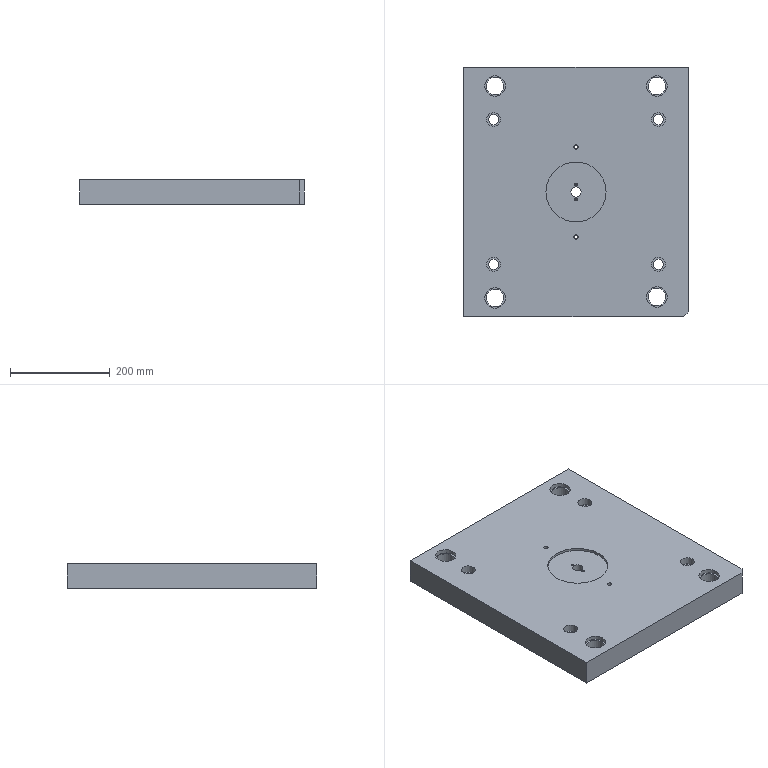Part | STEP file | SL2-MOLD_id730_xmt_txt | 1 solid | 46 faces | box 450 x 500 x 50 mm | volume 10885298 mm3 | cylinder 24 | plane 20 | cone 2 | commonest cylinder face diameters 20.5 x5 27.5 x4 35 x4 41 x4 5 x2 6 x2
STEP:
#1=CARTESIAN_POINT('',(-225.,-160.,136.));
#2=VERTEX_POINT('',#1);
#3=CARTESIAN_POINT('',(215.,-160.,136.));
#4=VERTEX_POINT('',#3);
#5=CARTESIAN_POINT('',(-130.,-160.,136.));
#6=DIRECTION('',(1.,0.,0.));
#7=VECTOR('',#6,1.);
#8=LINE('',#5,#7);
#9=EDGE_CURVE('',#2,#4,#8,.T.);
#10=ORIENTED_EDGE('',*,*,#9,.T.);
#11=CARTESIAN_POINT('',(215.,-160.,186.));
#12=VERTEX_POINT('',#11);
#13=CARTESIAN_POINT('',(215.,-160.,186.));
#14=DIRECTION('',(0.,0.,1.));
#15=VECTOR('',#14,1.);
#16=LINE('',#13,#15);
#17=EDGE_CURVE('',#4,#12,#16,.T.);
#18=ORIENTED_EDGE('',*,*,#17,.T.);
#19=CARTESIAN_POINT('',(-225.,-160.,186.));
#20=VERTEX_POINT('',#19);
#21=CARTESIAN_POINT('',(-130.,-160.,186.));
#22=DIRECTION('',(1.,0.,0.));
#23=VECTOR('',#22,1.);
#24=LINE('',#21,#23);
#25=EDGE_CURVE('',#20,#12,#24,.T.);
#26=ORIENTED_EDGE('',*,*,#25,.F.);
#27=CARTESIAN_POINT('',(-225.,-160.,186.));
#28=DIRECTION('',(0.,0.,-1.));
#29=VECTOR('',#28,1.);
#30=LINE('',#27,#29);
#31=EDGE_CURVE('',#20,#2,#30,.T.);
#32=ORIENTED_EDGE('',*,*,#31,.T.);
#33=EDGE_LOOP('',(#10,#18,#26,#32));
#34=FACE_OUTER_BOUND('',#33,.T.);
#35=CARTESIAN_POINT('',(-130.,-160.,186.));
#36=DIRECTION('',(0.,1.,0.));
#37=DIRECTION('',(0.,0.,1.));
#38=AXIS2_PLACEMENT_3D('',#35,#36,#37);
#39=PLANE('',#38);
#40=ADVANCED_FACE('',(#34),#39,.F.);
#41=CARTESIAN_POINT('',(225.,340.,186.));
#42=VERTEX_POINT('',#41);
#43=CARTESIAN_POINT('',(225.,-150.,186.));
#44=VERTEX_POINT('',#43);
#45=CARTESIAN_POINT('',(225.,-110.,186.));
#46=DIRECTION('',(0.,-1.,0.));
#47=VECTOR('',#46,1.);
#48=LINE('',#45,#47);
#49=EDGE_CURVE('',#42,#44,#48,.T.);
#50=ORIENTED_EDGE('',*,*,#49,.T.);
#51=CARTESIAN_POINT('',(225.,-150.,136.));
#52=VERTEX_POINT('',#51);
#53=CARTESIAN_POINT('',(225.,-150.,136.));
#54=DIRECTION('',(0.,0.,-1.));
#55=VECTOR('',#54,1.);
#56=LINE('',#53,#55);
#57=EDGE_CURVE('',#44,#52,#56,.T.);
#58=ORIENTED_EDGE('',*,*,#57,.T.);
#59=CARTESIAN_POINT('',(225.,340.,136.));
#60=VERTEX_POINT('',#59);
#61=CARTESIAN_POINT('',(225.,-110.,136.));
#62=DIRECTION('',(0.,-1.,0.));
#63=VECTOR('',#62,1.);
#64=LINE('',#61,#63);
#65=EDGE_CURVE('',#60,#52,#64,.T.);
#66=ORIENTED_EDGE('',*,*,#65,.F.);
#67=CARTESIAN_POINT('',(225.,340.,186.));
#68=DIRECTION('',(0.,0.,-1.));
#69=VECTOR('',#68,1.);
#70=LINE('',#67,#69);
#71=EDGE_CURVE('',#42,#60,#70,.T.);
#72=ORIENTED_EDGE('',*,*,#71,.F.);
#73=EDGE_LOOP('',(#50,#58,#66,#72));
#74=FACE_OUTER_BOUND('',#73,.T.);
#75=CARTESIAN_POINT('',(225.,-110.,186.));
#76=DIRECTION('',(1.,0.,0.));
#77=DIRECTION('',(0.,0.,-1.));
#78=AXIS2_PLACEMENT_3D('',#75,#76,#77);
#79=PLANE('',#78);
#80=ADVANCED_FACE('',(#74),#79,.T.);
#81=CARTESIAN_POINT('',(-225.,340.,136.));
#82=VERTEX_POINT('',#81);
#83=CARTESIAN_POINT('',(1.401,340.,136.));
#84=DIRECTION('',(-1.,0.,0.));
#85=VECTOR('',#84,1.);
#86=LINE('',#83,#85);
#87=EDGE_CURVE('',#60,#82,#86,.T.);
#88=ORIENTED_EDGE('',*,*,#87,.T.);
#89=CARTESIAN_POINT('',(-225.,340.,186.));
#90=VERTEX_POINT('',#89);
#91=CARTESIAN_POINT('',(-225.,340.,186.));
#92=DIRECTION('',(0.,0.,-1.));
#93=VECTOR('',#92,1.);
#94=LINE('',#91,#93);
#95=EDGE_CURVE('',#90,#82,#94,.T.);
#96=ORIENTED_EDGE('',*,*,#95,.F.);
#97=CARTESIAN_POINT('',(1.401,340.,186.));
#98=DIRECTION('',(-1.,0.,0.));
#99=VECTOR('',#98,1.);
#100=LINE('',#97,#99);
#101=EDGE_CURVE('',#42,#90,#100,.T.);
#102=ORIENTED_EDGE('',*,*,#101,.F.);
#103=ORIENTED_EDGE('',*,*,#71,.T.);
#104=EDGE_LOOP('',(#88,#96,#102,#103));
#105=FACE_OUTER_BOUND('',#104,.T.);
#106=CARTESIAN_POINT('',(1.401,340.,186.));
#107=DIRECTION('',(0.,-1.,0.));
#108=DIRECTION('',(0.,0.,-1.));
#109=AXIS2_PLACEMENT_3D('',#106,#107,#108);
#110=PLANE('',#109);
#111=ADVANCED_FACE('',(#105),#110,.F.);
#112=CARTESIAN_POINT('',(-225.,-4.582,136.));
#113=DIRECTION('',(0.,1.,0.));
#114=VECTOR('',#113,1.);
#115=LINE('',#112,#114);
#116=EDGE_CURVE('',#2,#82,#115,.T.);
#117=ORIENTED_EDGE('',*,*,#116,.F.);
#118=ORIENTED_EDGE('',*,*,#31,.F.);
#119=CARTESIAN_POINT('',(-225.,-4.582,186.));
#120=DIRECTION('',(0.,1.,0.));
#121=VECTOR('',#120,1.);
#122=LINE('',#119,#121);
#123=EDGE_CURVE('',#20,#90,#122,.T.);
#124=ORIENTED_EDGE('',*,*,#123,.T.);
#125=ORIENTED_EDGE('',*,*,#95,.T.);
#126=EDGE_LOOP('',(#117,#118,#124,#125));
#127=FACE_OUTER_BOUND('',#126,.T.);
#128=CARTESIAN_POINT('',(-225.,-4.582,186.));
#129=DIRECTION('',(-1.,0.,0.));
#130=DIRECTION('',(0.,0.,1.));
#131=AXIS2_PLACEMENT_3D('',#128,#129,#130);
#132=PLANE('',#131);
#133=ADVANCED_FACE('',(#127),#132,.T.);
#134=CARTESIAN_POINT('',(178.75,235.,186.));
#135=VERTEX_POINT('',#134);
#136=CARTESIAN_POINT('',(165.,235.,186.));
#137=DIRECTION('',(0.,0.,1.));
#138=DIRECTION('',(1.,0.,0.));
#139=AXIS2_PLACEMENT_3D('',#136,#137,#138);
#140=CIRCLE('',#139,13.75);
#141=EDGE_CURVE('',#135,#135,#140,.T.);
#142=ORIENTED_EDGE('',*,*,#141,.F.);
#143=EDGE_LOOP('',(#142));
#144=FACE_BOUND('',#143,.T.);
#145=CARTESIAN_POINT('',(-151.25,235.,186.));
#146=VERTEX_POINT('',#145);
#147=CARTESIAN_POINT('',(-165.,235.,186.));
#148=DIRECTION('',(0.,0.,1.));
#149=DIRECTION('',(1.,0.,0.));
#150=AXIS2_PLACEMENT_3D('',#147,#148,#149);
#151=CIRCLE('',#150,13.75);
#152=EDGE_CURVE('',#146,#146,#151,.T.);
#153=ORIENTED_EDGE('',*,*,#152,.F.);
#154=EDGE_LOOP('',(#153));
#155=FACE_BOUND('',#154,.T.);
#156=CARTESIAN_POINT('',(-151.25,-55.,186.));
#157=VERTEX_POINT('',#156);
#158=CARTESIAN_POINT('',(-165.,-55.,186.));
#159=DIRECTION('',(0.,0.,1.));
#160=DIRECTION('',(1.,0.,0.));
#161=AXIS2_PLACEMENT_3D('',#158,#159,#160);
#162=CIRCLE('',#161,13.75);
#163=EDGE_CURVE('',#157,#157,#162,.T.);
#164=ORIENTED_EDGE('',*,*,#163,.F.);
#165=EDGE_LOOP('',(#164));
#166=FACE_BOUND('',#165,.T.);
#167=CARTESIAN_POINT('',(178.75,-55.,186.));
#168=VERTEX_POINT('',#167);
#169=CARTESIAN_POINT('',(165.,-55.,186.));
#170=DIRECTION('',(0.,0.,1.));
#171=DIRECTION('',(1.,0.,0.));
#172=AXIS2_PLACEMENT_3D('',#169,#170,#171);
#173=CIRCLE('',#172,13.75);
#174=EDGE_CURVE('',#168,#168,#173,.T.);
#175=ORIENTED_EDGE('',*,*,#174,.F.);
#176=EDGE_LOOP('',(#175));
#177=FACE_BOUND('',#176,.T.);
#178=CARTESIAN_POINT('',(4.25,0.,186.));
#179=VERTEX_POINT('',#178);
#180=CARTESIAN_POINT('',(0.,0.,186.));
#181=DIRECTION('',(0.,0.,-1.));
#182=DIRECTION('',(1.,0.,0.));
#183=AXIS2_PLACEMENT_3D('',#180,#181,#182);
#184=CIRCLE('',#183,4.25);
#185=EDGE_CURVE('',#179,#179,#184,.T.);
#186=ORIENTED_EDGE('',*,*,#185,.T.);
#187=EDGE_LOOP('',(#186));
#188=FACE_BOUND('',#187,.T.);
#189=CARTESIAN_POINT('',(4.25,180.,186.));
#190=VERTEX_POINT('',#189);
#191=CARTESIAN_POINT('',(0.,180.,186.));
#192=DIRECTION('',(0.,0.,-1.));
#193=DIRECTION('',(1.,0.,0.));
#194=AXIS2_PLACEMENT_3D('',#191,#192,#193);
#195=CIRCLE('',#194,4.25);
#196=EDGE_CURVE('',#190,#190,#195,.T.);
#197=ORIENTED_EDGE('',*,*,#196,.T.);
#198=EDGE_LOOP('',(#197));
#199=FACE_BOUND('',#198,.T.);
#200=CARTESIAN_POINT('',(60.25,90.,186.));
#201=VERTEX_POINT('',#200);
#202=CARTESIAN_POINT('',(0.,90.,186.));
#203=DIRECTION('',(0.,0.,1.));
#204=DIRECTION('',(1.,0.,0.));
#205=AXIS2_PLACEMENT_3D('',#202,#203,#204);
#206=CIRCLE('',#205,60.25);
#207=EDGE_CURVE('',#201,#201,#206,.T.);
#208=ORIENTED_EDGE('',*,*,#207,.F.);
#209=EDGE_LOOP('',(#208));
#210=FACE_BOUND('',#209,.T.);
#211=CARTESIAN_POINT('',(-141.5,-122.,186.));
#212=VERTEX_POINT('',#211);
#213=CARTESIAN_POINT('',(-162.,-122.,186.));
#214=DIRECTION('',(0.,0.,-1.));
#215=DIRECTION('',(1.,0.,0.));
#216=AXIS2_PLACEMENT_3D('',#213,#214,#215);
#217=CIRCLE('',#216,20.5);
#218=EDGE_CURVE('',#212,#212,#217,.T.);
#219=ORIENTED_EDGE('',*,*,#218,.T.);
#220=EDGE_LOOP('',(#219));
#221=FACE_BOUND('',#220,.T.);
#222=CARTESIAN_POINT('',(182.5,-120.,186.));
#223=VERTEX_POINT('',#222);
#224=CARTESIAN_POINT('',(162.,-120.,186.));
#225=DIRECTION('',(0.,0.,-1.));
#226=DIRECTION('',(1.,0.,0.));
#227=AXIS2_PLACEMENT_3D('',#224,#225,#226);
#228=CIRCLE('',#227,20.5);
#229=EDGE_CURVE('',#223,#223,#228,.T.);
#230=ORIENTED_EDGE('',*,*,#229,.T.);
#231=EDGE_LOOP('',(#230));
#232=FACE_BOUND('',#231,.T.);
#233=CARTESIAN_POINT('',(182.5,302.,186.));
#234=VERTEX_POINT('',#233);
#235=CARTESIAN_POINT('',(162.,302.,186.));
#236=DIRECTION('',(0.,0.,-1.));
#237=DIRECTION('',(1.,0.,0.));
#238=AXIS2_PLACEMENT_3D('',#235,#236,#237);
#239=CIRCLE('',#238,20.5);
#240=EDGE_CURVE('',#234,#234,#239,.T.);
#241=ORIENTED_EDGE('',*,*,#240,.T.);
#242=EDGE_LOOP('',(#241));
#243=FACE_BOUND('',#242,.T.);
#244=CARTESIAN_POINT('',(-141.5,302.,186.));
#245=VERTEX_POINT('',#244);
#246=CARTESIAN_POINT('',(-162.,302.,186.));
#247=DIRECTION('',(0.,0.,-1.));
#248=DIRECTION('',(1.,0.,0.));
#249=AXIS2_PLACEMENT_3D('',#246,#247,#248);
#250=CIRCLE('',#249,20.5);
#251=EDGE_CURVE('',#245,#245,#250,.T.);
#252=ORIENTED_EDGE('',*,*,#251,.T.);
#253=EDGE_LOOP('',(#252));
#254=FACE_BOUND('',#253,.T.);
#255=ORIENTED_EDGE('',*,*,#25,.T.);
#256=CARTESIAN_POINT('',(185.909,-189.091,186.));
#257=DIRECTION('',(0.7071,0.7071,0.));
#258=VECTOR('',#257,1.);
#259=LINE('',#256,#258);
#260=EDGE_CURVE('',#12,#44,#259,.T.);
#261=ORIENTED_EDGE('',*,*,#260,.T.);
#262=ORIENTED_EDGE('',*,*,#49,.F.);
#263=ORIENTED_EDGE('',*,*,#101,.T.);
#264=ORIENTED_EDGE('',*,*,#123,.F.);
#265=EDGE_LOOP('',(#255,#261,#262,#263,#264));
#266=FACE_BOUND('',#265,.T.);
#267=CARTESIAN_POINT('',(1.401,-4.582,186.));
#268=DIRECTION('',(0.,0.,1.));
#269=DIRECTION('',(1.,0.,0.));
#270=AXIS2_PLACEMENT_3D('',#267,#268,#269);
#271=PLANE('',#270);
#272=ADVANCED_FACE('',(#144,#155,#166,#177,#188,#199,#210,#221,#232,#243,#254,#266),#271,.T.);
#273=CARTESIAN_POINT('',(175.25,235.,136.));
#274=VERTEX_POINT('',#273);
#275=CARTESIAN_POINT('',(165.,235.,136.));
#276=DIRECTION('',(0.,0.,-1.));
#277=DIRECTION('',(1.,0.,0.));
#278=AXIS2_PLACEMENT_3D('',#275,#276,#277);
#279=CIRCLE('',#278,10.25);
#280=EDGE_CURVE('',#274,#274,#279,.T.);
#281=ORIENTED_EDGE('',*,*,#280,.F.);
#282=EDGE_LOOP('',(#281));
#283=FACE_BOUND('',#282,.T.);
#284=CARTESIAN_POINT('',(-154.75,235.,136.));
#285=VERTEX_POINT('',#284);
#286=CARTESIAN_POINT('',(-165.,235.,136.));
#287=DIRECTION('',(0.,0.,-1.));
#288=DIRECTION('',(1.,0.,0.));
#289=AXIS2_PLACEMENT_3D('',#286,#287,#288);
#290=CIRCLE('',#289,10.25);
#291=EDGE_CURVE('',#285,#285,#290,.T.);
#292=ORIENTED_EDGE('',*,*,#291,.F.);
#293=EDGE_LOOP('',(#292));
#294=FACE_BOUND('',#293,.T.);
#295=CARTESIAN_POINT('',(-154.75,-55.,136.));
#296=VERTEX_POINT('',#295);
#297=CARTESIAN_POINT('',(-165.,-55.,136.));
#298=DIRECTION('',(0.,0.,-1.));
#299=DIRECTION('',(1.,0.,0.));
#300=AXIS2_PLACEMENT_3D('',#297,#298,#299);
#301=CIRCLE('',#300,10.25);
#302=EDGE_CURVE('',#296,#296,#301,.T.);
#303=ORIENTED_EDGE('',*,*,#302,.F.);
#304=EDGE_LOOP('',(#303));
#305=FACE_BOUND('',#304,.T.);
#306=CARTESIAN_POINT('',(175.25,-55.,136.));
#307=VERTEX_POINT('',#306);
#308=CARTESIAN_POINT('',(165.,-55.,136.));
#309=DIRECTION('',(0.,0.,-1.));
#310=DIRECTION('',(1.,0.,0.));
#311=AXIS2_PLACEMENT_3D('',#308,#309,#310);
#312=CIRCLE('',#311,10.25);
#313=EDGE_CURVE('',#307,#307,#312,.T.);
#314=ORIENTED_EDGE('',*,*,#313,.F.);
#315=EDGE_LOOP('',(#314));
#316=FACE_BOUND('',#315,.T.);
#317=CARTESIAN_POINT('',(3.,0.,136.));
#318=VERTEX_POINT('',#317);
#319=CARTESIAN_POINT('',(0.,0.,136.));
#320=DIRECTION('',(0.,0.,-1.));
#321=DIRECTION('',(1.,0.,0.));
#322=AXIS2_PLACEMENT_3D('',#319,#320,#321);
#323=CIRCLE('',#322,3.);
#324=EDGE_CURVE('',#318,#318,#323,.T.);
#325=ORIENTED_EDGE('',*,*,#324,.F.);
#326=EDGE_LOOP('',(#325));
#327=FACE_BOUND('',#326,.T.);
#328=CARTESIAN_POINT('',(3.,180.,136.));
#329=VERTEX_POINT('',#328);
#330=CARTESIAN_POINT('',(0.,180.,136.));
#331=DIRECTION('',(0.,0.,-1.));
#332=DIRECTION('',(1.,0.,0.));
#333=AXIS2_PLACEMENT_3D('',#330,#331,#332);
#334=CIRCLE('',#333,3.);
#335=EDGE_CURVE('',#329,#329,#334,.T.);
#336=ORIENTED_EDGE('',*,*,#335,.F.);
#337=EDGE_LOOP('',(#336));
#338=FACE_BOUND('',#337,.T.);
#339=CARTESIAN_POINT('',(10.25,90.,136.));
#340=VERTEX_POINT('',#339);
#341=CARTESIAN_POINT('',(0.,90.,136.));
#342=DIRECTION('',(0.,0.,-1.));
#343=DIRECTION('',(1.,0.,0.));
#344=AXIS2_PLACEMENT_3D('',#341,#342,#343);
#345=CIRCLE('',#344,10.25);
#346=EDGE_CURVE('',#340,#340,#345,.T.);
#347=ORIENTED_EDGE('',*,*,#346,.F.);
#348=EDGE_LOOP('',(#347));
#349=FACE_BOUND('',#348,.T.);
#350=CARTESIAN_POINT('',(-144.5,-122.,136.));
#351=VERTEX_POINT('',#350);
#352=CARTESIAN_POINT('',(-162.,-122.,136.));
#353=DIRECTION('',(0.,0.,-1.));
#354=DIRECTION('',(1.,0.,0.));
#355=AXIS2_PLACEMENT_3D('',#352,#353,#354);
#356=CIRCLE('',#355,17.5);
#357=EDGE_CURVE('',#351,#351,#356,.T.);
#358=ORIENTED_EDGE('',*,*,#357,.F.);
#359=EDGE_LOOP('',(#358));
#360=FACE_BOUND('',#359,.T.);
#361=CARTESIAN_POINT('',(179.5,-120.,136.));
#362=VERTEX_POINT('',#361);
#363=CARTESIAN_POINT('',(162.,-120.,136.));
#364=DIRECTION('',(0.,0.,-1.));
#365=DIRECTION('',(1.,0.,0.));
#366=AXIS2_PLACEMENT_3D('',#363,#364,#365);
#367=CIRCLE('',#366,17.5);
#368=EDGE_CURVE('',#362,#362,#367,.T.);
#369=ORIENTED_EDGE('',*,*,#368,.F.);
#370=EDGE_LOOP('',(#369));
#371=FACE_BOUND('',#370,.T.);
#372=CARTESIAN_POINT('',(179.5,302.,136.));
#373=VERTEX_POINT('',#372);
#374=CARTESIAN_POINT('',(162.,302.,136.));
#375=DIRECTION('',(0.,0.,-1.));
#376=DIRECTION('',(1.,0.,0.));
#377=AXIS2_PLACEMENT_3D('',#374,#375,#376);
#378=CIRCLE('',#377,17.5);
#379=EDGE_CURVE('',#373,#373,#378,.T.);
#380=ORIENTED_EDGE('',*,*,#379,.F.);
#381=EDGE_LOOP('',(#380));
#382=FACE_BOUND('',#381,.T.);
#383=CARTESIAN_POINT('',(-144.5,302.,136.));
#384=VERTEX_POINT('',#383);
#385=CARTESIAN_POINT('',(-162.,302.,136.));
#386=DIRECTION('',(0.,0.,-1.));
#387=DIRECTION('',(1.,0.,0.));
#388=AXIS2_PLACEMENT_3D('',#385,#386,#387);
#389=CIRCLE('',#388,17.5);
#390=EDGE_CURVE('',#384,#384,#389,.T.);
#391=ORIENTED_EDGE('',*,*,#390,.F.);
#392=EDGE_LOOP('',(#391));
#393=FACE_BOUND('',#392,.T.);
#394=ORIENTED_EDGE('',*,*,#65,.T.);
#395=CARTESIAN_POINT('',(225.,-150.,136.));
#396=DIRECTION('',(-0.7071,-0.7071,0.));
#397=VECTOR('',#396,1.);
#398=LINE('',#395,#397);
#399=EDGE_CURVE('',#52,#4,#398,.T.);
#400=ORIENTED_EDGE('',*,*,#399,.T.);
#401=ORIENTED_EDGE('',*,*,#9,.F.);
#402=ORIENTED_EDGE('',*,*,#116,.T.);
#403=ORIENTED_EDGE('',*,*,#87,.F.);
#404=EDGE_LOOP('',(#394,#400,#401,#402,#403));
#405=FACE_BOUND('',#404,.T.);
#406=CARTESIAN_POINT('',(1.401,-4.582,136.));
#407=DIRECTION('',(0.,0.,1.));
#408=DIRECTION('',(1.,0.,0.));
#409=AXIS2_PLACEMENT_3D('',#406,#407,#408);
#410=PLANE('',#409);
#411=ADVANCED_FACE('',(#283,#294,#305,#316,#327,#338,#349,#360,#371,#382,#393,#405),#410,.F.);
#412=ORIENTED_EDGE('',*,*,#260,.F.);
#413=ORIENTED_EDGE('',*,*,#17,.F.);
#414=ORIENTED_EDGE('',*,*,#399,.F.);
#415=ORIENTED_EDGE('',*,*,#57,.F.);
#416=EDGE_LOOP('',(#412,#413,#414,#415));
#417=FACE_OUTER_BOUND('',#416,.T.);
#418=CARTESIAN_POINT('',(225.,-150.,186.));
#419=DIRECTION('',(0.7071,-0.7071,0.));
#420=DIRECTION('',(0.,0.,1.));
#421=AXIS2_PLACEMENT_3D('',#418,#419,#420);
#422=PLANE('',#421);
#423=ADVANCED_FACE('',(#417),#422,.T.);
#424=ORIENTED_EDGE('',*,*,#251,.F.);
#425=EDGE_LOOP('',(#424));
#426=FACE_BOUND('',#425,.T.);
#427=CARTESIAN_POINT('',(-141.5,302.,178.));
#428=VERTEX_POINT('',#427);
#429=CARTESIAN_POINT('',(-162.,302.,178.));
#430=DIRECTION('',(0.,0.,-1.));
#431=DIRECTION('',(1.,0.,0.));
#432=AXIS2_PLACEMENT_3D('',#429,#430,#431);
#433=CIRCLE('',#432,20.5);
#434=EDGE_CURVE('',#428,#428,#433,.T.);
#435=ORIENTED_EDGE('',*,*,#434,.T.);
#436=EDGE_LOOP('',(#435));
#437=FACE_BOUND('',#436,.T.);
#438=CARTESIAN_POINT('',(-162.,302.,208.));
#439=DIRECTION('',(0.,0.,-1.));
#440=DIRECTION('',(-1.,0.,0.));
#441=AXIS2_PLACEMENT_3D('',#438,#439,#440);
#442=CYLINDRICAL_SURFACE('',#441,20.5);
#443=ADVANCED_FACE('',(#426,#437),#442,.F.);
#444=CARTESIAN_POINT('',(-179.5,302.,178.));
#445=VERTEX_POINT('',#444);
#446=CARTESIAN_POINT('',(-162.,302.,178.));
#447=DIRECTION('',(0.,0.,-1.));
#448=DIRECTION('',(-1.,0.,0.));
#449=AXIS2_PLACEMENT_3D('',#446,#447,#448);
#450=CIRCLE('',#449,17.5);
#451=EDGE_CURVE('',#445,#445,#450,.T.);
#452=ORIENTED_EDGE('',*,*,#451,.T.);
#453=EDGE_LOOP('',(#452));
#454=FACE_BOUND('',#453,.T.);
#455=ORIENTED_EDGE('',*,*,#434,.F.);
#456=EDGE_LOOP('',(#455));
#457=FACE_BOUND('',#456,.T.);
#458=CARTESIAN_POINT('',(-162.,302.,178.));
#459=DIRECTION('',(0.,0.,1.));
#460=DIRECTION('',(1.,0.,0.));
#461=AXIS2_PLACEMENT_3D('',#458,#459,#460);
#462=PLANE('',#461);
#463=ADVANCED_FACE('',(#454,#457),#462,.T.);
#464=ORIENTED_EDGE('',*,*,#240,.F.);
#465=EDGE_LOOP('',(#464));
#466=FACE_BOUND('',#465,.T.);
#467=CARTESIAN_POINT('',(182.5,302.,178.));
#468=VERTEX_POINT('',#467);
#469=CARTESIAN_POINT('',(162.,302.,178.));
#470=DIRECTION('',(0.,0.,-1.));
#471=DIRECTION('',(1.,0.,0.));
#472=AXIS2_PLACEMENT_3D('',#469,#470,#471);
#473=CIRCLE('',#472,20.5);
#474=EDGE_CURVE('',#468,#468,#473,.T.);
#475=ORIENTED_EDGE('',*,*,#474,.T.);
#476=EDGE_LOOP('',(#475));
#477=FACE_BOUND('',#476,.T.);
#478=CARTESIAN_POINT('',(162.,302.,208.));
#479=DIRECTION('',(0.,0.,-1.));
#480=DIRECTION('',(-1.,0.,0.));
#481=AXIS2_PLACEMENT_3D('',#478,#479,#480);
#482=CYLINDRICAL_SURFACE('',#481,20.5);
#483=ADVANCED_FACE('',(#466,#477),#482,.F.);
#484=CARTESIAN_POINT('',(144.5,302.,178.));
#485=VERTEX_POINT('',#484);
#486=CARTESIAN_POINT('',(162.,302.,178.));
#487=DIRECTION('',(0.,0.,-1.));
#488=DIRECTION('',(-1.,0.,0.));
#489=AXIS2_PLACEMENT_3D('',#486,#487,#488);
#490=CIRCLE('',#489,17.5);
#491=EDGE_CURVE('',#485,#485,#490,.T.);
#492=ORIENTED_EDGE('',*,*,#491,.T.);
#493=EDGE_LOOP('',(#492));
#494=FACE_BOUND('',#493,.T.);
#495=ORIENTED_EDGE('',*,*,#474,.F.);
#496=EDGE_LOOP('',(#495));
#497=FACE_BOUND('',#496,.T.);
#498=CARTESIAN_POINT('',(162.,302.,178.));
#499=DIRECTION('',(0.,0.,1.));
#500=DIRECTION('',(1.,0.,0.));
#501=AXIS2_PLACEMENT_3D('',#498,#499,#500);
#502=PLANE('',#501);
#503=ADVANCED_FACE('',(#494,#497),#502,.T.);
#504=ORIENTED_EDGE('',*,*,#229,.F.);
#505=EDGE_LOOP('',(#504));
#506=FACE_BOUND('',#505,.T.);
#507=CARTESIAN_POINT('',(182.5,-120.,178.));
#508=VERTEX_POINT('',#507);
#509=CARTESIAN_POINT('',(162.,-120.,178.));
#510=DIRECTION('',(0.,0.,-1.));
#511=DIRECTION('',(1.,0.,0.));
#512=AXIS2_PLACEMENT_3D('',#509,#510,#511);
#513=CIRCLE('',#512,20.5);
#514=EDGE_CURVE('',#508,#508,#513,.T.);
#515=ORIENTED_EDGE('',*,*,#514,.T.);
#516=EDGE_LOOP('',(#515));
#517=FACE_BOUND('',#516,.T.);
#518=CARTESIAN_POINT('',(162.,-120.,208.));
#519=DIRECTION('',(0.,0.,-1.));
#520=DIRECTION('',(-1.,0.,0.));
#521=AXIS2_PLACEMENT_3D('',#518,#519,#520);
#522=CYLINDRICAL_SURFACE('',#521,20.5);
#523=ADVANCED_FACE('',(#506,#517),#522,.F.);
#524=CARTESIAN_POINT('',(144.5,-120.,178.));
#525=VERTEX_POINT('',#524);
#526=CARTESIAN_POINT('',(162.,-120.,178.));
#527=DIRECTION('',(0.,0.,-1.));
#528=DIRECTION('',(-1.,0.,0.));
#529=AXIS2_PLACEMENT_3D('',#526,#527,#528);
#530=CIRCLE('',#529,17.5);
#531=EDGE_CURVE('',#525,#525,#530,.T.);
#532=ORIENTED_EDGE('',*,*,#531,.T.);
#533=EDGE_LOOP('',(#532));
#534=FACE_BOUND('',#533,.T.);
#535=ORIENTED_EDGE('',*,*,#514,.F.);
#536=EDGE_LOOP('',(#535));
#537=FACE_BOUND('',#536,.T.);
#538=CARTESIAN_POINT('',(162.,-120.,178.));
#539=DIRECTION('',(0.,0.,1.));
#540=DIRECTION('',(1.,0.,0.));
#541=AXIS2_PLACEMENT_3D('',#538,#539,#540);
#542=PLANE('',#541);
#543=ADVANCED_FACE('',(#534,#537),#542,.T.);
#544=ORIENTED_EDGE('',*,*,#218,.F.);
#545=EDGE_LOOP('',(#544));
#546=FACE_BOUND('',#545,.T.);
#547=CARTESIAN_POINT('',(-141.5,-122.,178.));
#548=VERTEX_POINT('',#547);
#549=CARTESIAN_POINT('',(-162.,-122.,178.));
#550=DIRECTION('',(0.,0.,-1.));
#551=DIRECTION('',(1.,0.,0.));
#552=AXIS2_PLACEMENT_3D('',#549,#550,#551);
#553=CIRCLE('',#552,20.5);
#554=EDGE_CURVE('',#548,#548,#553,.T.);
#555=ORIENTED_EDGE('',*,*,#554,.T.);
#556=EDGE_LOOP('',(#555));
#557=FACE_BOUND('',#556,.T.);
#558=CARTESIAN_POINT('',(-162.,-122.,208.));
#559=DIRECTION('',(0.,0.,-1.));
#560=DIRECTION('',(-1.,0.,0.));
#561=AXIS2_PLACEMENT_3D('',#558,#559,#560);
#562=CYLINDRICAL_SURFACE('',#561,20.5);
#563=ADVANCED_FACE('',(#546,#557),#562,.F.);
#564=CARTESIAN_POINT('',(-179.5,-122.,178.));
#565=VERTEX_POINT('',#564);
#566=CARTESIAN_POINT('',(-162.,-122.,178.));
#567=DIRECTION('',(0.,0.,-1.));
#568=DIRECTION('',(-1.,0.,0.));
#569=AXIS2_PLACEMENT_3D('',#566,#567,#568);
#570=CIRCLE('',#569,17.5);
#571=EDGE_CURVE('',#565,#565,#570,.T.);
#572=ORIENTED_EDGE('',*,*,#571,.T.);
#573=EDGE_LOOP('',(#572));
#574=FACE_BOUND('',#573,.T.);
#575=ORIENTED_EDGE('',*,*,#554,.F.);
#576=EDGE_LOOP('',(#575));
#577=FACE_BOUND('',#576,.T.);
#578=CARTESIAN_POINT('',(-162.,-122.,178.));
#579=DIRECTION('',(0.,0.,1.));
#580=DIRECTION('',(1.,0.,0.));
#581=AXIS2_PLACEMENT_3D('',#578,#579,#580);
#582=PLANE('',#581);
#583=ADVANCED_FACE('',(#574,#577),#582,.T.);
#584=ORIENTED_EDGE('',*,*,#451,.F.);
#585=EDGE_LOOP('',(#584));
#586=FACE_BOUND('',#585,.T.);
#587=ORIENTED_EDGE('',*,*,#390,.T.);
#588=EDGE_LOOP('',(#587));
#589=FACE_BOUND('',#588,.T.);
#590=CARTESIAN_POINT('',(-162.,302.,3221.8));
#591=DIRECTION('',(0.,0.,-1.));
#592=DIRECTION('',(-1.,0.,0.));
#593=AXIS2_PLACEMENT_3D('',#590,#591,#592);
#594=CYLINDRICAL_SURFACE('',#593,17.5);
#595=ADVANCED_FACE('',(#586,#589),#594,.F.);
#596=ORIENTED_EDGE('',*,*,#491,.F.);
#597=EDGE_LOOP('',(#596));
#598=FACE_BOUND('',#597,.T.);
#599=ORIENTED_EDGE('',*,*,#379,.T.);
#600=EDGE_LOOP('',(#599));
#601=FACE_BOUND('',#600,.T.);
#602=CARTESIAN_POINT('',(162.,302.,3221.8));
#603=DIRECTION('',(0.,0.,-1.));
#604=DIRECTION('',(-1.,0.,0.));
#605=AXIS2_PLACEMENT_3D('',#602,#603,#604);
#606=CYLINDRICAL_SURFACE('',#605,17.5);
#607=ADVANCED_FACE('',(#598,#601),#606,.F.);
#608=ORIENTED_EDGE('',*,*,#531,.F.);
#609=EDGE_LOOP('',(#608));
#610=FACE_BOUND('',#609,.T.);
#611=ORIENTED_EDGE('',*,*,#368,.T.);
#612=EDGE_LOOP('',(#611));
#613=FACE_BOUND('',#612,.T.);
#614=CARTESIAN_POINT('',(162.,-120.,3221.8));
#615=DIRECTION('',(0.,0.,-1.));
#616=DIRECTION('',(-1.,0.,0.));
#617=AXIS2_PLACEMENT_3D('',#614,#615,#616);
#618=CYLINDRICAL_SURFACE('',#617,17.5);
#619=ADVANCED_FACE('',(#610,#613),#618,.F.);
#620=ORIENTED_EDGE('',*,*,#571,.F.);
#621=EDGE_LOOP('',(#620));
#622=FACE_BOUND('',#621,.T.);
#623=ORIENTED_EDGE('',*,*,#357,.T.);
#624=EDGE_LOOP('',(#623));
#625=FACE_BOUND('',#624,.T.);
#626=CARTESIAN_POINT('',(-162.,-122.,3221.8));
#627=DIRECTION('',(0.,0.,-1.));
#628=DIRECTION('',(-1.,0.,0.));
#629=AXIS2_PLACEMENT_3D('',#626,#627,#628);
#630=CYLINDRICAL_SURFACE('',#629,17.5);
#631=ADVANCED_FACE('',(#622,#625),#630,.F.);
#632=CARTESIAN_POINT('',(-2.5,75.,181.));
#633=VERTEX_POINT('',#632);
#634=CARTESIAN_POINT('',(0.,75.,181.));
#635=DIRECTION('',(0.,0.,-1.));
#636=DIRECTION('',(-1.,0.,0.));
#637=AXIS2_PLACEMENT_3D('',#634,#635,#636);
#638=CIRCLE('',#637,2.5);
#639=EDGE_CURVE('',#633,#633,#638,.T.);
#640=ORIENTED_EDGE('',*,*,#639,.T.);
#641=EDGE_LOOP('',(#640));
#642=FACE_BOUND('',#641,.T.);
#643=CARTESIAN_POINT('',(-2.5,105.,181.));
#644=VERTEX_POINT('',#643);
#645=CARTESIAN_POINT('',(0.,105.,181.));
#646=DIRECTION('',(0.,0.,-1.));
#647=DIRECTION('',(-1.,0.,0.));
#648=AXIS2_PLACEMENT_3D('',#645,#646,#647);
#649=CIRCLE('',#648,2.5);
#650=EDGE_CURVE('',#644,#644,#649,.T.);
#651=ORIENTED_EDGE('',*,*,#650,.T.);
#652=EDGE_LOOP('',(#651));
#653=FACE_BOUND('',#652,.T.);
#654=CARTESIAN_POINT('',(-10.25,90.,181.));
#655=VERTEX_POINT('',#654);
#656=CARTESIAN_POINT('',(0.,90.,181.));
#657=DIRECTION('',(0.,0.,-1.));
#658=DIRECTION('',(-1.,0.,0.));
#659=AXIS2_PLACEMENT_3D('',#656,#657,#658);
#660=CIRCLE('',#659,10.25);
#661=EDGE_CURVE('',#655,#655,#660,.T.);
#662=ORIENTED_EDGE('',*,*,#661,.T.);
#663=EDGE_LOOP('',(#662));
#664=FACE_BOUND('',#663,.T.);
#665=CARTESIAN_POINT('',(-60.25,90.,181.));
#666=VERTEX_POINT('',#665);
#667=CARTESIAN_POINT('',(0.,90.,181.));
#668=DIRECTION('',(0.,0.,-1.));
#669=DIRECTION('',(-1.,0.,0.));
#670=AXIS2_PLACEMENT_3D('',#667,#668,#669);
#671=CIRCLE('',#670,60.25);
#672=EDGE_CURVE('',#666,#666,#671,.T.);
#673=ORIENTED_EDGE('',*,*,#672,.F.);
#674=EDGE_LOOP('',(#673));
#675=FACE_BOUND('',#674,.T.);
#676=CARTESIAN_POINT('',(0.,90.,181.));
#677=DIRECTION('',(0.,0.,-1.));
#678=DIRECTION('',(1.,0.,0.));
#679=AXIS2_PLACEMENT_3D('',#676,#677,#678);
#680=PLANE('',#679);
#681=ADVANCED_FACE('',(#642,#653,#664,#675),#680,.F.);
#682=ORIENTED_EDGE('',*,*,#207,.T.);
#683=EDGE_LOOP('',(#682));
#684=FACE_BOUND('',#683,.T.);
#685=ORIENTED_EDGE('',*,*,#672,.T.);
#686=EDGE_LOOP('',(#685));
#687=FACE_BOUND('',#686,.T.);
#688=CARTESIAN_POINT('',(0.,90.,374.55));
#689=DIRECTION('',(0.,0.,-1.));
#690=DIRECTION('',(-1.,0.,0.));
#691=AXIS2_PLACEMENT_3D('',#688,#689,#690);
#692=CYLINDRICAL_SURFACE('',#691,60.25);
#693=ADVANCED_FACE('',(#684,#687),#692,.F.);
#694=ORIENTED_EDGE('',*,*,#661,.F.);
#695=EDGE_LOOP('',(#694));
#696=FACE_BOUND('',#695,.T.);
#697=ORIENTED_EDGE('',*,*,#346,.T.);
#698=EDGE_LOOP('',(#697));
#699=FACE_BOUND('',#698,.T.);
#700=CARTESIAN_POINT('',(0.,90.,810.846));
#701=DIRECTION('',(0.,0.,-1.));
#702=DIRECTION('',(-1.,0.,0.));
#703=AXIS2_PLACEMENT_3D('',#700,#701,#702);
#704=CYLINDRICAL_SURFACE('',#703,10.25);
#705=ADVANCED_FACE('',(#696,#699),#704,.F.);
#706=CARTESIAN_POINT('',(0.,102.5,174.));
#707=VERTEX_POINT('',#706);
#708=CARTESIAN_POINT('',(0.,105.,174.));
#709=DIRECTION('',(0.,0.,1.));
#710=DIRECTION('',(0.,-1.,0.));
#711=AXIS2_PLACEMENT_3D('',#708,#709,#710);
#712=CIRCLE('',#711,2.5);
#713=EDGE_CURVE('',#707,#707,#712,.T.);
#714=ORIENTED_EDGE('',*,*,#713,.F.);
#715=EDGE_LOOP('',(#714));
#716=FACE_BOUND('',#715,.T.);
#717=ORIENTED_EDGE('',*,*,#650,.F.);
#718=EDGE_LOOP('',(#717));
#719=FACE_BOUND('',#718,.T.);
#720=CARTESIAN_POINT('',(0.,105.,179.5));
#721=DIRECTION('',(0.,0.,-1.));
#722=DIRECTION('',(0.,-1.,0.));
#723=AXIS2_PLACEMENT_3D('',#720,#721,#722);
#724=CYLINDRICAL_SURFACE('',#723,2.5);
#725=ADVANCED_FACE('',(#716,#719),#724,.F.);
#726=ORIENTED_EDGE('',*,*,#713,.T.);
#727=EDGE_LOOP('',(#726));
#728=FACE_BOUND('',#727,.T.);
#729=CARTESIAN_POINT('',(0.,103.,173.5));
#730=VERTEX_POINT('',#729);
#731=CARTESIAN_POINT('',(0.,105.,173.5));
#732=DIRECTION('',(0.,0.,-1.));
#733=DIRECTION('',(0.,-1.,0.));
#734=AXIS2_PLACEMENT_3D('',#731,#732,#733);
#735=CIRCLE('',#734,2.);
#736=EDGE_CURVE('',#730,#730,#735,.T.);
#737=ORIENTED_EDGE('',*,*,#736,.T.);
#738=EDGE_LOOP('',(#737));
#739=FACE_BOUND('',#738,.T.);
#740=CARTESIAN_POINT('',(0.,105.,173.5));
#741=DIRECTION('',(0.,0.,1.));
#742=DIRECTION('',(0.,1.,0.));
#743=AXIS2_PLACEMENT_3D('',#740,#741,#742);
#744=CONICAL_SURFACE('',#743,2.,45.);
#745=ADVANCED_FACE('',(#728,#739),#744,.F.);
#746=ORIENTED_EDGE('',*,*,#736,.F.);
#747=EDGE_LOOP('',(#746));
#748=FACE_OUTER_BOUND('',#747,.T.);
#749=CARTESIAN_POINT('',(0.,105.,173.5));
#750=DIRECTION('',(0.,0.,-1.));
#751=DIRECTION('',(0.,-1.,0.));
#752=AXIS2_PLACEMENT_3D('',#749,#750,#751);
#753=PLANE('',#752);
#754=ADVANCED_FACE('',(#748),#753,.F.);
#755=CARTESIAN_POINT('',(0.,72.5,174.));
#756=VERTEX_POINT('',#755);
#757=CARTESIAN_POINT('',(0.,75.,174.));
#758=DIRECTION('',(0.,0.,1.));
#759=DIRECTION('',(0.,-1.,0.));
#760=AXIS2_PLACEMENT_3D('',#757,#758,#759);
#761=CIRCLE('',#760,2.5);
#762=EDGE_CURVE('',#756,#756,#761,.T.);
#763=ORIENTED_EDGE('',*,*,#762,.F.);
#764=EDGE_LOOP('',(#763));
#765=FACE_BOUND('',#764,.T.);
#766=ORIENTED_EDGE('',*,*,#639,.F.);
#767=EDGE_LOOP('',(#766));
#768=FACE_BOUND('',#767,.T.);
#769=CARTESIAN_POINT('',(0.,75.,179.5));
#770=DIRECTION('',(0.,0.,-1.));
#771=DIRECTION('',(0.,-1.,0.));
#772=AXIS2_PLACEMENT_3D('',#769,#770,#771);
#773=CYLINDRICAL_SURFACE('',#772,2.5);
#774=ADVANCED_FACE('',(#765,#768),#773,.F.);
#775=ORIENTED_EDGE('',*,*,#762,.T.);
#776=EDGE_LOOP('',(#775));
#777=FACE_BOUND('',#776,.T.);
#778=CARTESIAN_POINT('',(0.,73.,173.5));
#779=VERTEX_POINT('',#778);
#780=CARTESIAN_POINT('',(0.,75.,173.5));
#781=DIRECTION('',(0.,0.,-1.));
#782=DIRECTION('',(0.,-1.,0.));
#783=AXIS2_PLACEMENT_3D('',#780,#781,#782);
#784=CIRCLE('',#783,2.);
#785=EDGE_CURVE('',#779,#779,#784,.T.);
#786=ORIENTED_EDGE('',*,*,#785,.T.);
#787=EDGE_LOOP('',(#786));
#788=FACE_BOUND('',#787,.T.);
#789=CARTESIAN_POINT('',(0.,75.,173.5));
#790=DIRECTION('',(0.,0.,1.));
#791=DIRECTION('',(0.,1.,0.));
#792=AXIS2_PLACEMENT_3D('',#789,#790,#791);
#793=CONICAL_SURFACE('',#792,2.,45.);
#794=ADVANCED_FACE('',(#777,#788),#793,.F.);
#795=ORIENTED_EDGE('',*,*,#785,.F.);
#796=EDGE_LOOP('',(#795));
#797=FACE_OUTER_BOUND('',#796,.T.);
#798=CARTESIAN_POINT('',(0.,75.,173.5));
#799=DIRECTION('',(0.,0.,-1.));
#800=DIRECTION('',(0.,-1.,0.));
#801=AXIS2_PLACEMENT_3D('',#798,#799,#800);
#802=PLANE('',#801);
#803=ADVANCED_FACE('',(#797),#802,.F.);
#804=ORIENTED_EDGE('',*,*,#196,.F.);
#805=EDGE_LOOP('',(#804));
#806=FACE_BOUND('',#805,.T.);
#807=CARTESIAN_POINT('',(4.25,180.,160.));
#808=VERTEX_POINT('',#807);
#809=CARTESIAN_POINT('',(0.,180.,160.));
#810=DIRECTION('',(0.,0.,-1.));
#811=DIRECTION('',(1.,0.,0.));
#812=AXIS2_PLACEMENT_3D('',#809,#810,#811);
#813=CIRCLE('',#812,4.25);
#814=EDGE_CURVE('',#808,#808,#813,.T.);
#815=ORIENTED_EDGE('',*,*,#814,.T.);
#816=EDGE_LOOP('',(#815));
#817=FACE_BOUND('',#816,.T.);
#818=CARTESIAN_POINT('',(0.,180.,180.));
#819=DIRECTION('',(0.,0.,-1.));
#820=DIRECTION('',(-1.,0.,0.));
#821=AXIS2_PLACEMENT_3D('',#818,#819,#820);
#822=CYLINDRICAL_SURFACE('',#821,4.25);
#823=ADVANCED_FACE('',(#806,#817),#822,.F.);
#824=CARTESIAN_POINT('',(-3.,180.,160.));
#825=VERTEX_POINT('',#824);
#826=CARTESIAN_POINT('',(0.,180.,160.));
#827=DIRECTION('',(0.,0.,-1.));
#828=DIRECTION('',(-1.,0.,0.));
#829=AXIS2_PLACEMENT_3D('',#826,#827,#828);
#830=CIRCLE('',#829,3.);
#831=EDGE_CURVE('',#825,#825,#830,.T.);
#832=ORIENTED_EDGE('',*,*,#831,.T.);
#833=EDGE_LOOP('',(#832));
#834=FACE_BOUND('',#833,.T.);
#835=ORIENTED_EDGE('',*,*,#814,.F.);
#836=EDGE_LOOP('',(#835));
#837=FACE_BOUND('',#836,.T.);
#838=CARTESIAN_POINT('',(0.,180.,160.));
#839=DIRECTION('',(0.,0.,1.));
#840=DIRECTION('',(1.,0.,0.));
#841=AXIS2_PLACEMENT_3D('',#838,#839,#840);
#842=PLANE('',#841);
#843=ADVANCED_FACE('',(#834,#837),#842,.T.);
#844=ORIENTED_EDGE('',*,*,#185,.F.);
#845=EDGE_LOOP('',(#844));
#846=FACE_BOUND('',#845,.T.);
#847=CARTESIAN_POINT('',(4.25,0.,160.));
#848=VERTEX_POINT('',#847);
#849=CARTESIAN_POINT('',(0.,0.,160.));
#850=DIRECTION('',(0.,0.,-1.));
#851=DIRECTION('',(1.,0.,0.));
#852=AXIS2_PLACEMENT_3D('',#849,#850,#851);
#853=CIRCLE('',#852,4.25);
#854=EDGE_CURVE('',#848,#848,#853,.T.);
#855=ORIENTED_EDGE('',*,*,#854,.T.);
#856=EDGE_LOOP('',(#855));
#857=FACE_BOUND('',#856,.T.);
#858=CARTESIAN_POINT('',(0.,0.,180.));
#859=DIRECTION('',(0.,0.,-1.));
#860=DIRECTION('',(-1.,0.,0.));
#861=AXIS2_PLACEMENT_3D('',#858,#859,#860);
#862=CYLINDRICAL_SURFACE('',#861,4.25);
#863=ADVANCED_FACE('',(#846,#857),#862,.F.);
#864=CARTESIAN_POINT('',(-3.,0.,160.));
#865=VERTEX_POINT('',#864);
#866=CARTESIAN_POINT('',(0.,0.,160.));
#867=DIRECTION('',(0.,0.,-1.));
#868=DIRECTION('',(-1.,0.,0.));
#869=AXIS2_PLACEMENT_3D('',#866,#867,#868);
#870=CIRCLE('',#869,3.);
#871=EDGE_CURVE('',#865,#865,#870,.T.);
#872=ORIENTED_EDGE('',*,*,#871,.T.);
#873=EDGE_LOOP('',(#872));
#874=FACE_BOUND('',#873,.T.);
#875=ORIENTED_EDGE('',*,*,#854,.F.);
#876=EDGE_LOOP('',(#875));
#877=FACE_BOUND('',#876,.T.);
#878=CARTESIAN_POINT('',(0.,0.,160.));
#879=DIRECTION('',(0.,0.,1.));
#880=DIRECTION('',(1.,0.,0.));
#881=AXIS2_PLACEMENT_3D('',#878,#879,#880);
#882=PLANE('',#881);
#883=ADVANCED_FACE('',(#874,#877),#882,.T.);
#884=ORIENTED_EDGE('',*,*,#831,.F.);
#885=EDGE_LOOP('',(#884));
#886=FACE_BOUND('',#885,.T.);
#887=ORIENTED_EDGE('',*,*,#335,.T.);
#888=EDGE_LOOP('',(#887));
#889=FACE_BOUND('',#888,.T.);
#890=CARTESIAN_POINT('',(0.,180.,658.4));
#891=DIRECTION('',(0.,0.,-1.));
#892=DIRECTION('',(-1.,0.,0.));
#893=AXIS2_PLACEMENT_3D('',#890,#891,#892);
#894=CYLINDRICAL_SURFACE('',#893,3.);
#895=ADVANCED_FACE('',(#886,#889),#894,.F.);
#896=ORIENTED_EDGE('',*,*,#871,.F.);
#897=EDGE_LOOP('',(#896));
#898=FACE_BOUND('',#897,.T.);
#899=ORIENTED_EDGE('',*,*,#324,.T.);
#900=EDGE_LOOP('',(#899));
#901=FACE_BOUND('',#900,.T.);
#902=CARTESIAN_POINT('',(0.,0.,658.4));
#903=DIRECTION('',(0.,0.,-1.));
#904=DIRECTION('',(-1.,0.,0.));
#905=AXIS2_PLACEMENT_3D('',#902,#903,#904);
#906=CYLINDRICAL_SURFACE('',#905,3.);
#907=ADVANCED_FACE('',(#898,#901),#906,.F.);
#908=ORIENTED_EDGE('',*,*,#174,.T.);
#909=EDGE_LOOP('',(#908));
#910=FACE_BOUND('',#909,.T.);
#911=CARTESIAN_POINT('',(151.25,-55.,171.));
#912=VERTEX_POINT('',#911);
#913=CARTESIAN_POINT('',(165.,-55.,171.));
#914=DIRECTION('',(0.,0.,-1.));
#915=DIRECTION('',(-1.,0.,0.));
#916=AXIS2_PLACEMENT_3D('',#913,#914,#915);
#917=CIRCLE('',#916,13.75);
#918=EDGE_CURVE('',#912,#912,#917,.T.);
#919=ORIENTED_EDGE('',*,*,#918,.T.);
#920=EDGE_LOOP('',(#919));
#921=FACE_BOUND('',#920,.T.);
#922=CARTESIAN_POINT('',(165.,-55.,204.));
#923=DIRECTION('',(0.,0.,-1.));
#924=DIRECTION('',(-1.,0.,0.));
#925=AXIS2_PLACEMENT_3D('',#922,#923,#924);
#926=CYLINDRICAL_SURFACE('',#925,13.75);
#927=ADVANCED_FACE('',(#910,#921),#926,.F.);
#928=ORIENTED_EDGE('',*,*,#163,.T.);
#929=EDGE_LOOP('',(#928));
#930=FACE_BOUND('',#929,.T.);
#931=CARTESIAN_POINT('',(-178.75,-55.,171.));
#932=VERTEX_POINT('',#931);
#933=CARTESIAN_POINT('',(-165.,-55.,171.));
#934=DIRECTION('',(0.,0.,-1.));
#935=DIRECTION('',(-1.,0.,0.));
#936=AXIS2_PLACEMENT_3D('',#933,#934,#935);
#937=CIRCLE('',#936,13.75);
#938=EDGE_CURVE('',#932,#932,#937,.T.);
#939=ORIENTED_EDGE('',*,*,#938,.T.);
#940=EDGE_LOOP('',(#939));
#941=FACE_BOUND('',#940,.T.);
#942=CARTESIAN_POINT('',(-165.,-55.,204.));
#943=DIRECTION('',(0.,0.,-1.));
#944=DIRECTION('',(-1.,0.,0.));
#945=AXIS2_PLACEMENT_3D('',#942,#943,#944);
#946=CYLINDRICAL_SURFACE('',#945,13.75);
#947=ADVANCED_FACE('',(#930,#941),#946,.F.);
#948=ORIENTED_EDGE('',*,*,#152,.T.);
#949=EDGE_LOOP('',(#948));
#950=FACE_BOUND('',#949,.T.);
#951=CARTESIAN_POINT('',(-178.75,235.,171.));
#952=VERTEX_POINT('',#951);
#953=CARTESIAN_POINT('',(-165.,235.,171.));
#954=DIRECTION('',(0.,0.,-1.));
#955=DIRECTION('',(-1.,0.,0.));
#956=AXIS2_PLACEMENT_3D('',#953,#954,#955);
#957=CIRCLE('',#956,13.75);
#958=EDGE_CURVE('',#952,#952,#957,.T.);
#959=ORIENTED_EDGE('',*,*,#958,.T.);
#960=EDGE_LOOP('',(#959));
#961=FACE_BOUND('',#960,.T.);
#962=CARTESIAN_POINT('',(-165.,235.,204.));
#963=DIRECTION('',(0.,0.,-1.));
#964=DIRECTION('',(-1.,0.,0.));
#965=AXIS2_PLACEMENT_3D('',#962,#963,#964);
#966=CYLINDRICAL_SURFACE('',#965,13.75);
#967=ADVANCED_FACE('',(#950,#961),#966,.F.);
#968=ORIENTED_EDGE('',*,*,#141,.T.);
#969=EDGE_LOOP('',(#968));
#970=FACE_BOUND('',#969,.T.);
#971=CARTESIAN_POINT('',(151.25,235.,171.));
#972=VERTEX_POINT('',#971);
#973=CARTESIAN_POINT('',(165.,235.,171.));
#974=DIRECTION('',(0.,0.,-1.));
#975=DIRECTION('',(-1.,0.,0.));
#976=AXIS2_PLACEMENT_3D('',#973,#974,#975);
#977=CIRCLE('',#976,13.75);
#978=EDGE_CURVE('',#972,#972,#977,.T.);
#979=ORIENTED_EDGE('',*,*,#978,.T.);
#980=EDGE_LOOP('',(#979));
#981=FACE_BOUND('',#980,.T.);
#982=CARTESIAN_POINT('',(165.,235.,204.));
#983=DIRECTION('',(0.,0.,-1.));
#984=DIRECTION('',(-1.,0.,0.));
#985=AXIS2_PLACEMENT_3D('',#982,#983,#984);
#986=CYLINDRICAL_SURFACE('',#985,13.75);
#987=ADVANCED_FACE('',(#970,#981),#986,.F.);
#988=CARTESIAN_POINT('',(154.75,-55.,171.));
#989=VERTEX_POINT('',#988);
#990=CARTESIAN_POINT('',(165.,-55.,171.));
#991=DIRECTION('',(0.,0.,-1.));
#992=DIRECTION('',(-1.,0.,0.));
#993=AXIS2_PLACEMENT_3D('',#990,#991,#992);
#994=CIRCLE('',#993,10.25);
#995=EDGE_CURVE('',#989,#989,#994,.T.);
#996=ORIENTED_EDGE('',*,*,#995,.F.);
#997=EDGE_LOOP('',(#996));
#998=FACE_BOUND('',#997,.T.);
#999=ORIENTED_EDGE('',*,*,#313,.T.);
#1000=EDGE_LOOP('',(#999));
#1001=FACE_BOUND('',#1000,.T.);
#1002=CARTESIAN_POINT('',(165.,-55.,153.5));
#1003=DIRECTION('',(0.,0.,-1.));
#1004=DIRECTION('',(1.,0.,0.));
#1005=AXIS2_PLACEMENT_3D('',#1002,#1003,#1004);
#1006=CYLINDRICAL_SURFACE('',#1005,10.25);
#1007=ADVANCED_FACE('',(#998,#1001),#1006,.F.);
#1008=ORIENTED_EDGE('',*,*,#995,.T.);
#1009=EDGE_LOOP('',(#1008));
#1010=FACE_BOUND('',#1009,.T.);
#1011=ORIENTED_EDGE('',*,*,#918,.F.);
#1012=EDGE_LOOP('',(#1011));
#1013=FACE_BOUND('',#1012,.T.);
#1014=CARTESIAN_POINT('',(165.,-55.,171.));
#1015=DIRECTION('',(0.,0.,-1.));
#1016=DIRECTION('',(1.,0.,0.));
#1017=AXIS2_PLACEMENT_3D('',#1014,#1015,#1016);
#1018=PLANE('',#1017);
#1019=ADVANCED_FACE('',(#1010,#1013),#1018,.F.);
#1020=CARTESIAN_POINT('',(-175.25,-55.,171.));
#1021=VERTEX_POINT('',#1020);
#1022=CARTESIAN_POINT('',(-165.,-55.,171.));
#1023=DIRECTION('',(0.,0.,-1.));
#1024=DIRECTION('',(-1.,0.,0.));
#1025=AXIS2_PLACEMENT_3D('',#1022,#1023,#1024);
#1026=CIRCLE('',#1025,10.25);
#1027=EDGE_CURVE('',#1021,#1021,#1026,.T.);
#1028=ORIENTED_EDGE('',*,*,#1027,.F.);
#1029=EDGE_LOOP('',(#1028));
#1030=FACE_BOUND('',#1029,.T.);
#1031=ORIENTED_EDGE('',*,*,#302,.T.);
#1032=EDGE_LOOP('',(#1031));
#1033=FACE_BOUND('',#1032,.T.);
#1034=CARTESIAN_POINT('',(-165.,-55.,153.5));
#1035=DIRECTION('',(0.,0.,-1.));
#1036=DIRECTION('',(1.,0.,0.));
#1037=AXIS2_PLACEMENT_3D('',#1034,#1035,#1036);
#1038=CYLINDRICAL_SURFACE('',#1037,10.25);
#1039=ADVANCED_FACE('',(#1030,#1033),#1038,.F.);
#1040=ORIENTED_EDGE('',*,*,#1027,.T.);
#1041=EDGE_LOOP('',(#1040));
#1042=FACE_BOUND('',#1041,.T.);
#1043=ORIENTED_EDGE('',*,*,#938,.F.);
#1044=EDGE_LOOP('',(#1043));
#1045=FACE_BOUND('',#1044,.T.);
#1046=CARTESIAN_POINT('',(-165.,-55.,171.));
#1047=DIRECTION('',(0.,0.,-1.));
#1048=DIRECTION('',(1.,0.,0.));
#1049=AXIS2_PLACEMENT_3D('',#1046,#1047,#1048);
#1050=PLANE('',#1049);
#1051=ADVANCED_FACE('',(#1042,#1045),#1050,.F.);
#1052=CARTESIAN_POINT('',(-175.25,235.,171.));
#1053=VERTEX_POINT('',#1052);
#1054=CARTESIAN_POINT('',(-165.,235.,171.));
#1055=DIRECTION('',(0.,0.,-1.));
#1056=DIRECTION('',(-1.,0.,0.));
#1057=AXIS2_PLACEMENT_3D('',#1054,#1055,#1056);
#1058=CIRCLE('',#1057,10.25);
#1059=EDGE_CURVE('',#1053,#1053,#1058,.T.);
#1060=ORIENTED_EDGE('',*,*,#1059,.F.);
#1061=EDGE_LOOP('',(#1060));
#1062=FACE_BOUND('',#1061,.T.);
#1063=ORIENTED_EDGE('',*,*,#291,.T.);
#1064=EDGE_LOOP('',(#1063));
#1065=FACE_BOUND('',#1064,.T.);
#1066=CARTESIAN_POINT('',(-165.,235.,153.5));
#1067=DIRECTION('',(0.,0.,-1.));
#1068=DIRECTION('',(1.,0.,0.));
#1069=AXIS2_PLACEMENT_3D('',#1066,#1067,#1068);
#1070=CYLINDRICAL_SURFACE('',#1069,10.25);
#1071=ADVANCED_FACE('',(#1062,#1065),#1070,.F.);
#1072=ORIENTED_EDGE('',*,*,#1059,.T.);
#1073=EDGE_LOOP('',(#1072));
#1074=FACE_BOUND('',#1073,.T.);
#1075=ORIENTED_EDGE('',*,*,#958,.F.);
#1076=EDGE_LOOP('',(#1075));
#1077=FACE_BOUND('',#1076,.T.);
#1078=CARTESIAN_POINT('',(-165.,235.,171.));
#1079=DIRECTION('',(0.,0.,-1.));
#1080=DIRECTION('',(1.,0.,0.));
#1081=AXIS2_PLACEMENT_3D('',#1078,#1079,#1080);
#1082=PLANE('',#1081);
#1083=ADVANCED_FACE('',(#1074,#1077),#1082,.F.);
#1084=CARTESIAN_POINT('',(154.75,235.,171.));
#1085=VERTEX_POINT('',#1084);
#1086=CARTESIAN_POINT('',(165.,235.,171.));
#1087=DIRECTION('',(0.,0.,-1.));
#1088=DIRECTION('',(-1.,0.,0.));
#1089=AXIS2_PLACEMENT_3D('',#1086,#1087,#1088);
#1090=CIRCLE('',#1089,10.25);
#1091=EDGE_CURVE('',#1085,#1085,#1090,.T.);
#1092=ORIENTED_EDGE('',*,*,#1091,.F.);
#1093=EDGE_LOOP('',(#1092));
#1094=FACE_BOUND('',#1093,.T.);
#1095=ORIENTED_EDGE('',*,*,#280,.T.);
#1096=EDGE_LOOP('',(#1095));
#1097=FACE_BOUND('',#1096,.T.);
#1098=CARTESIAN_POINT('',(165.,235.,153.5));
#1099=DIRECTION('',(0.,0.,-1.));
#1100=DIRECTION('',(1.,0.,0.));
#1101=AXIS2_PLACEMENT_3D('',#1098,#1099,#1100);
#1102=CYLINDRICAL_SURFACE('',#1101,10.25);
#1103=ADVANCED_FACE('',(#1094,#1097),#1102,.F.);
#1104=ORIENTED_EDGE('',*,*,#1091,.T.);
#1105=EDGE_LOOP('',(#1104));
#1106=FACE_BOUND('',#1105,.T.);
#1107=ORIENTED_EDGE('',*,*,#978,.F.);
#1108=EDGE_LOOP('',(#1107));
#1109=FACE_BOUND('',#1108,.T.);
#1110=CARTESIAN_POINT('',(165.,235.,171.));
#1111=DIRECTION('',(0.,0.,-1.));
#1112=DIRECTION('',(1.,0.,0.));
#1113=AXIS2_PLACEMENT_3D('',#1110,#1111,#1112);
#1114=PLANE('',#1113);
#1115=ADVANCED_FACE('',(#1106,#1109),#1114,.F.);
#1116=CLOSED_SHELL('',(#40,#80,#111,#133,#272,#411,#423,#443,#463,#483,#503,#523,#543,#563,#583,#595,#607,#619,#631,#681,#693,#705,#725,#745,#754,#774,#794,#803,#823,#843,#863,#883,#895,#907,#927,#947,#967,#987,#1007,#1019,#1039,#1051,#1071,#1083,#1103,#1115));
#1117=MANIFOLD_SOLID_BREP('',#1116);
#1118=(LENGTH_UNIT()NAMED_UNIT(*)SI_UNIT(.MILLI.,.METRE.));
#1119=UNCERTAINTY_MEASURE_WITH_UNIT(LENGTH_MEASURE(0.00002),#1118,'','');
#1120=(NAMED_UNIT(*)PLANE_ANGLE_UNIT()SI_UNIT($,.RADIAN.));
#1121=PLANE_ANGLE_MEASURE_WITH_UNIT(PLANE_ANGLE_MEASURE(0.01745),#1120);
#1122=DIMENSIONAL_EXPONENTS(0.,0.,0.,0.,0.,0.,0.);
#1123=(CONVERSION_BASED_UNIT('DEGREE',#1121)NAMED_UNIT(#1122)PLANE_ANGLE_UNIT());
#1124=(NAMED_UNIT(*)SI_UNIT($,.STERADIAN.)SOLID_ANGLE_UNIT());
#1125=(GEOMETRIC_REPRESENTATION_CONTEXT(3)GLOBAL_UNCERTAINTY_ASSIGNED_CONTEXT((#1119))GLOBAL_UNIT_ASSIGNED_CONTEXT((#1118,#1123,#1124))REPRESENTATION_CONTEXT('',''));
#1126=ADVANCED_BREP_SHAPE_REPRESENTATION('',(#1117),#1125);